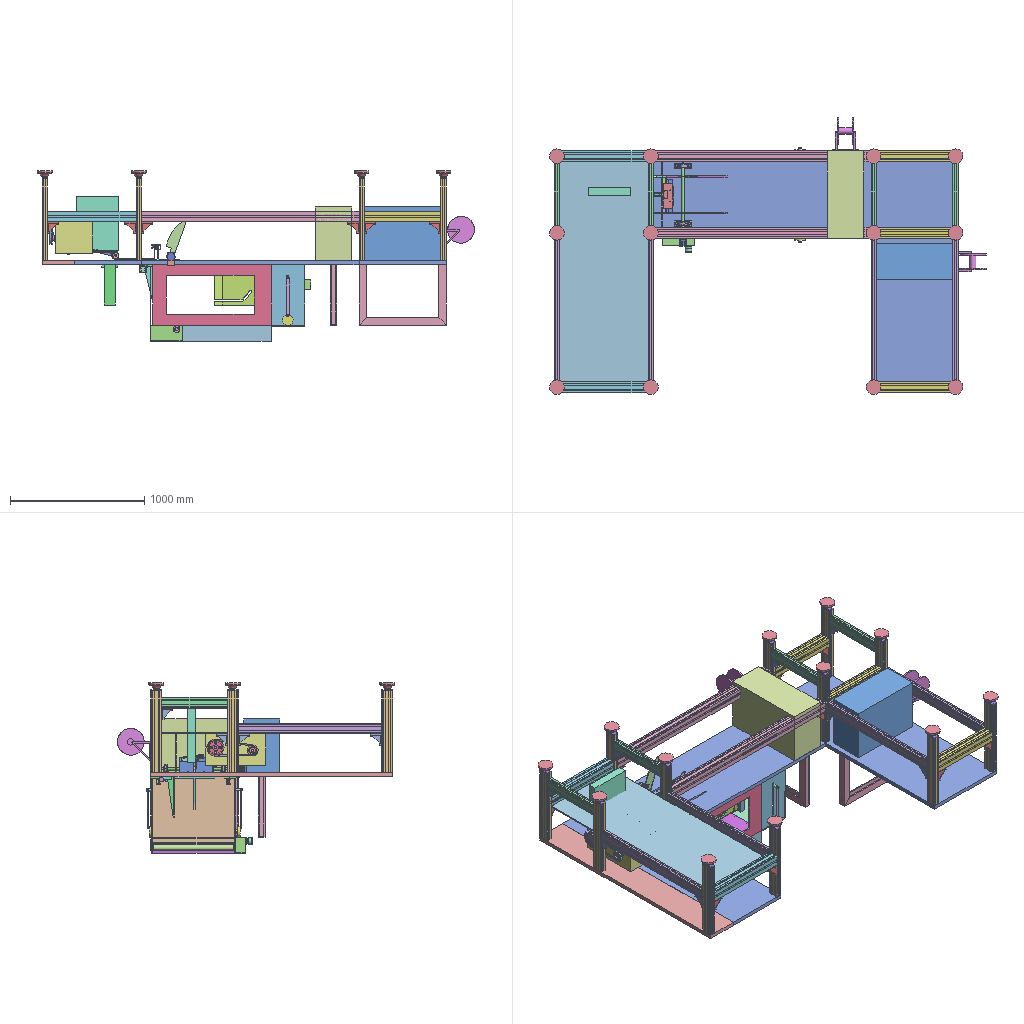Assembly | STEP file | 103 different items | 306 placed | box 3254 x 2065 x 1270 mm
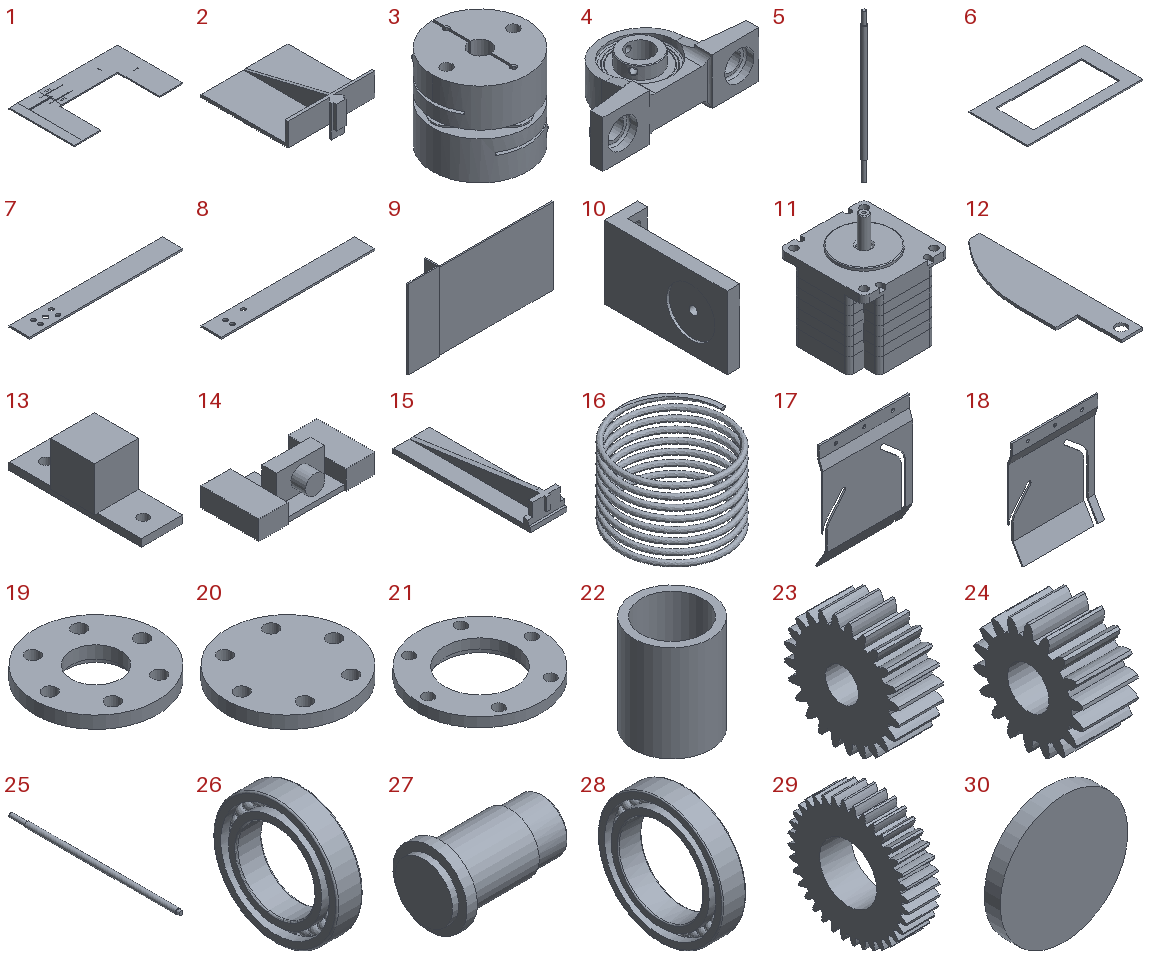Parts list (item | name | quantity | parent item | size | volume):
1 | Table top | x1 | in Assembly | 3010 x 1800 x 30 mm | 105133684 mm3
2 | tuishuban | x1 | in Assembly | 300 x 334 x 110 mm | 1327140 mm3
3 | Diaphragm coupling DEG01-D29-d6.35-e12 | x1 | in Assembly | 29 x 29 x 25.7 mm | 11994 mm3
4 | Pillow block bearing UCP204_D20 | x2 | in Assembly | 127 x 65 x 38 mm | 98212 mm3
5 | chuandongzhou | x1 | in Assembly | 20 x 20 x 596.6 mm | 161289 mm3
6 | ceban | x2 | in Assembly | 880 x 450 x 10 mm | 2061950 mm3
7 | zhiheceban1 | x1 | in Assembly | 900 x 120 x 10 mm | 1052932 mm3
8 | zhiheceban2 | x1 | in Assembly | 900 x 120 x 10 mm | 1066428 mm3
9 | zhihediban | x1 | in Assembly | 1150 x 120 x 626 mm | 7685600 mm3
10 | 57dianjijia | x1 | in Assembly | 26 x 96.5 x 57 mm | 58808 mm3
11 | 57bujindianji | x1 | in Assembly | 57 x 57 x 71.7 mm | 148752 mm3
12 | qianjiaozheban | x2 | in Assembly | 80 x 300 x 5 mm | 88356 mm3
13 | diancitie | x1 | in duizhongjigou | 30 x 90 x 35 mm | 39215 mm3
14 | duishubandingweicao | x1 | in duizhongjigou | 120 x 60 x 35 mm | 115212 mm3
15 | duizhongban | x1 | in duizhongjigou | 80 x 300 x 50 mm | 326800 mm3
16 | tanhuang | x1 | in duizhongjigou | - | 381.944 mm3
17 | gudingzhezhiban2 | x1 | in Assembly | 300 x 38.971 x 370 mm | 526356 mm3
18 | gudingzhezhiban1 | x1 | in Assembly | 300 x 39.641 x 372.5 mm | 530723 mm3
19 | zhouchenyagai1 | x4 | in Assembly | 40 x 40 x 6 mm | 4104 mm3
20 | zhouchenyagai2 | x3 | in Assembly | 40 x 40 x 6 mm | 4909 mm3
21 | zhouchenyagai3 | x1 | in Assembly | 51 x 51 x 6 mm | 5562 mm3
22 | dingjuguan | x4 | in Assembly | 20 x 20 x 25 mm | 2827 mm3
23 | spur gear_gb_GB - Spur gear 2M 24T 20PA 20FW ---S24A75H50L15.0N | x1 | in Assembly | 20 x 51.691 x 51.691 mm | 31658 mm3
24 | spur gear_gb_GB - Spur gear 2M 18T 20PA 20FW ---S18A75H50L15.0N | x2 | in Assembly | 20 x 39.557 x 40 mm | 16040 mm3
25 | tulunzhou | x1 | in Assembly | 20 x 672 x 20 mm | 200669 mm3
26 | deep groove ball bearings gb_Rolling bearings 61802 GB 276-94 | x7 | in Assembly | 5 x 24 x 24 mm | 1018 mm3
27 | zhou2 | x1 | in Assembly | 58 x 36 x 36 mm | 34937 mm3
28 | deep groove ball bearings gb_Rolling bearings 61805 GB 276-94 | x2 | in Assembly | 7 x 37 x 37 mm | 3011 mm3
29 | spur gear_gb_GB - Spur gear 2M 36T 20PA 20FW ---S36A75H50L36.0N | x1 | in Assembly | 20 x 75.809 x 75.809 mm | 59641 mm3
30 | zhoutaoφ36 | x1 | in Assembly | 48 x 9 x 48 mm | 11498 mm3
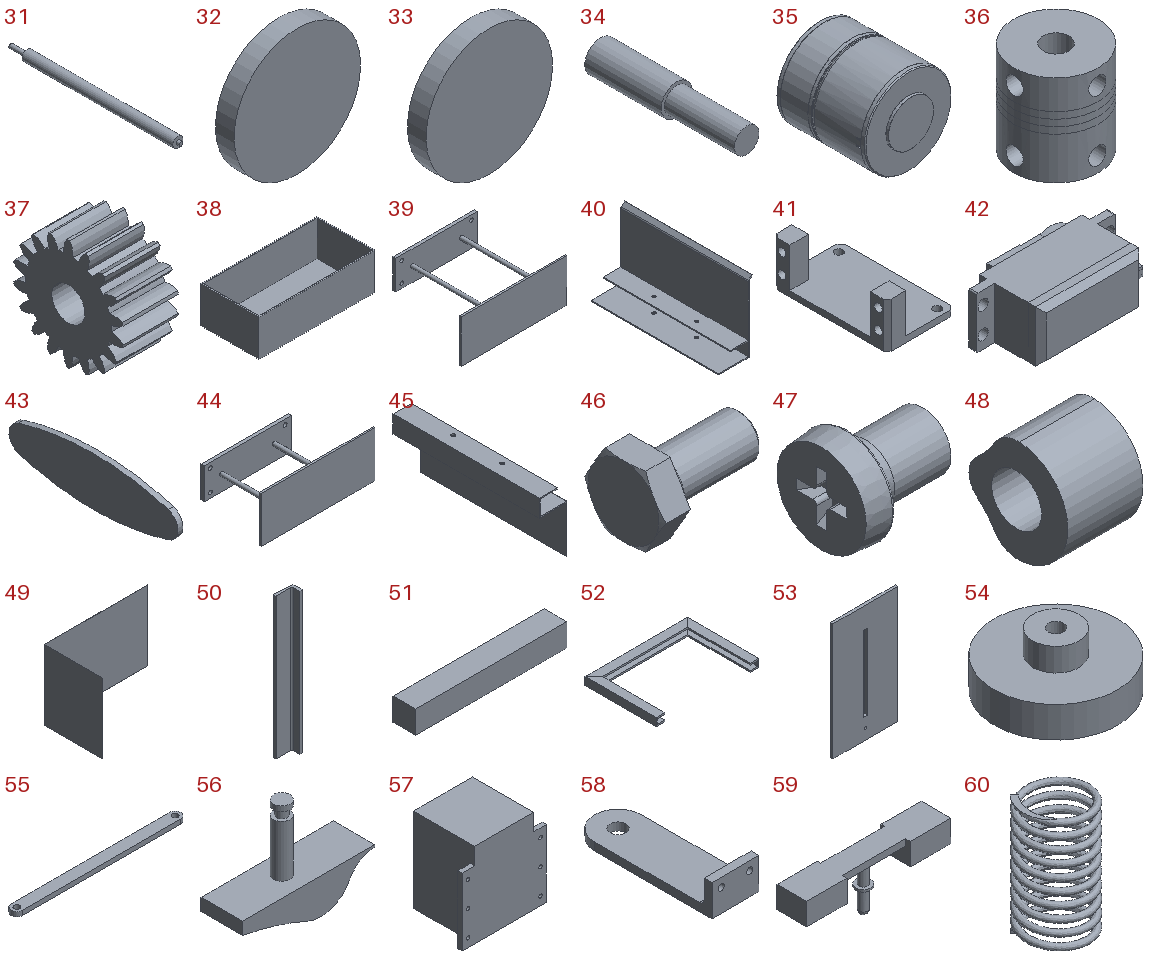31 | songzhizhou | x2 | in Assembly | 40 x 672 x 40 mm | 762386 mm3
32 | zhoutao_φ16 | x6 | in Assembly | 34 x 7 x 34 mm | 4705 mm3
33 | zhouchengai3 | x1 | in Assembly | 34 x 7 x 34 mm | 4705 mm3
34 | chilunshuruzhou | x1 | in Assembly | 15 x 71 x 15 mm | 10384 mm3
35 | zhiliudianji_Ratio 171 & 226 | x1 | in Assembly | 50 x 63.8 x 50 mm | 24472 mm3
36 | lianzhouqi | x1 | in Assembly | 19.5 x 19.5 x 21 mm | 4222 mm3
37 | spur gear_gb_GB - Spur gear 2M 18T 20PA 20FW ---S18A75H50L12.0N | x1 | in Assembly | 20 x 39.557 x 40 mm | 17312 mm3
38 | xiang | x1 | in Assembly | 240 x 120 x 75.5 mm | 239250 mm3
39 | zhijia | x1 | in zheshangye | 182 x 138 x 83.7 mm | 82026 mm3
40 | zheshangyeban | x1 | in zheshangye | 67 x 250 x 138.414 mm | 116601 mm3
41 | Servo fixing bracket-Y-middle | x2 | in Servo_left | 34.5 x 58 x 23 mm | 8576 mm3
42 | Huisheng 995 servo-Y | x2 | in Servo_left | 54 x 31.7 x 20 mm | 21472 mm3
43 | zheyetulun | x2 | in zheshangye, zhexiaye | 8 x 98.136 x 28.217 mm | 6682 mm3
44 | zhijia2 | x1 | in zhexiaye | 182 x 118 x 78.7 mm | 80895 mm3
45 | zhexiayeban | x1 | in zhexiaye | 49 x 250 x 110 mm | 92261 mm3
46 | hexagon head bolts-full thread gb_GB_FASTENER_BOLT_STBAB A M6X12-C | x8 | in zhexiaye, Assembly | 16.15 x 11.293 x 9.78 mm | 674.74 mm3
47 | cross recessed cheese head screws type a gb_GB_CROSS_SCREWS_TYPE135 M3X4-N | x10 | in zhexiaye | 5.4 x 4.982 x 4.982 mm | 52.121 mm3
48 | cuozhitulun | x1 | in Assembly | 30 x 39.5 x 40.969 mm | 25744 mm3
49 | zhi | x1 | in Assembly | 891 x 505.5 x 606 mm | 845626 mm3
50 | daozhiban | x1 | in Assembly | 80 x 45.5 x 606 mm | 689617 mm3
51 | jiazhi | x4 | in Assembly | 80 x 12 x 12 mm | 11520 mm3
52 | kunza | x2 | in Assembly | 650 x 450 x 50 mm | 1951319 mm3
53 | tieqianjijia | x1 | in Assembly | 250 x 10 x 450 mm | 1077815 mm3
54 | tieqianqubin | x2 | in Assembly | 80 x 80 x 48 mm | 111746 mm3
55 | tieqiangan | x2 | in Assembly | 300 x 20 x 8 mm | 46057 mm3
56 | tieqianhuakuai | x2 | in Assembly | 128 x 40 x 97.212 mm | 118551 mm3
57 | tieqiandianji | x2 | in Assembly | 100 x 72.5 x 123 mm | 526820 mm3
58 | tieqianzhizhu | x2 | in Assembly | 60 x 180 x 40 mm | 118454 mm3
59 | tieqiantou | x2 | in Assembly | 340 x 70 x 128 mm | 841793 mm3
60 | tieqiantanhuang | x1 | in Assembly | 21.623 x 21.623 x 40 mm | 1892 mm3
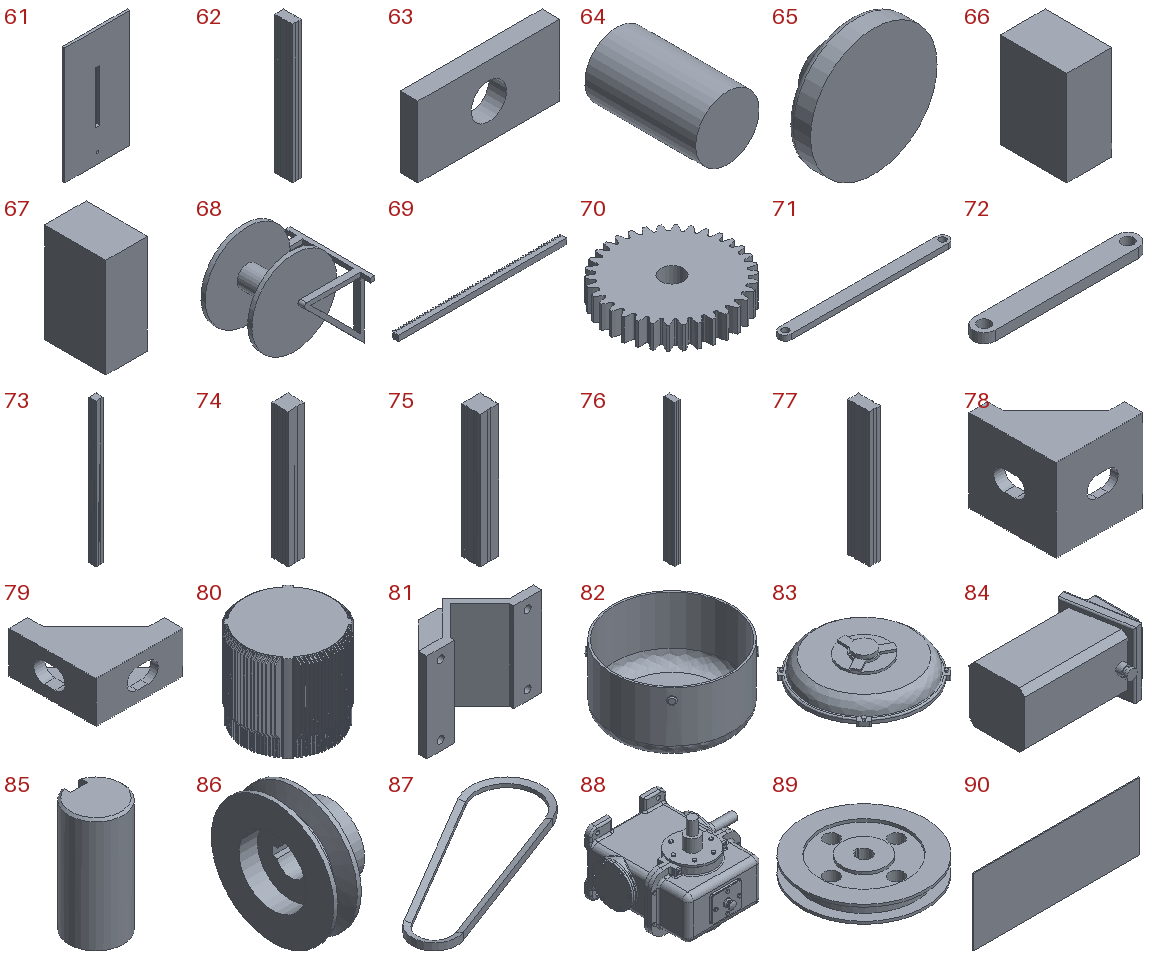61 | tieqianjijia2 | x1 | in Assembly | 250 x 10 x 450 mm | 1092215 mm3
62 | xingcai40x80x800 | x13 | in xingcaijiao | 40 x 80 x 609 mm | 1846488 mm3
63 | dianpian | x13 | in xingcaijiao | 80 x 10 x 40 mm | 28858 mm3
64 | dijiaolianjie | x13 | in xingcaijiao | 20 x 35 x 20 mm | 10996 mm3
65 | dijiao | x13 | in xingcaijiao | 110 x 46 x 110 mm | 258314 mm3
66 | kunzaxiang | x1 | in Assembly | 270 x 400 x 570 mm | 12312000 mm3
67 | kunzaxiang2 | x1 | in Assembly | 270 x 400 x 650 mm | 28248000 mm3
68 | daizhuantong | x2 | in Assembly | 250 x 200 x 250 mm | 976487 mm3
69 | rack spur rectangular_gb_GB - Rack-spur - rectangular 1.5M 20PA 10FW 10PH 300L---SAll | x2 | in Assembly | 300 x 11.5 x 10 mm | 29060 mm3
70 | Cylindrical gear 34_1.5 | x1 | in Assembly | 54 x 53.862 x 10 mm | 19460 mm3
71 | Connecting rod | x1 | in Assembly | 254.04 x 18 x 8 mm | 34769 mm3
72 | Crank | x1 | in Assembly | 136.8 x 18 x 8 mm | 17886 mm3
73 | xingcai80x80x1620 | x2 | in Assembly | 80 x 80 x 1620 mm | 10095840 mm3
74 | xingcai80x80x420 | x2 | in Assembly | 80 x 80 x 660 mm | 4113120 mm3
75 | xingcai80x80x570 | x3 | in Assembly | 80 x 80 x 570 mm | 3552240 mm3
76 | xingcai40x80x1070 | x4 | in Assembly | 40 x 80 x 1070 mm | 3244240 mm3
77 | xingcai40x80x490 | x4 | in Assembly | 40 x 80 x 490 mm | 1485680 mm3
78 | jiaoma80 | x14 | in Assembly | 84 x 84 x 80 mm | 134159 mm3
79 | jiaoma | x17 | in Assembly | 84 x 84 x 40 mm | 78299 mm3
80 | Y2_JZ_80_B_1.step 1 | x1 | in Three-phase asynchronous motor_B3_Y2-802-4_I_1 | 175 x 175 x 160 mm | 3332448 mm3
81 | Y2_DJ_80.step 2 | x1 | in Three-phase asynchronous motor_B3_Y2-802-4_I_1 | 165 x 80 x 128 mm | 452320 mm3
82 | Y2_FZ_80_1.step 3 | x1 | in Three-phase asynchronous motor_B3_Y2-802-4_I_1 | 171.5 x 171.5 x 90 mm | 182303 mm3
83 | Y2_B3_FL_80_1.step 4 | x1 | in Three-phase asynchronous motor_B3_Y2-802-4_I_1 | 157.5 x 157.5 x 35 mm | 429524 mm3
84 | Y2_JXH_80.step 5 | x1 | in Three-phase asynchronous motor_B3_Y2-802-4_I_1 | 145 x 87.322 x 78.75 mm | 651359 mm3
85 | Y2_SCZ_80_1.step 6 | x1 | in Three-phase asynchronous motor_B3_Y2-802-4_I_1 | 19 x 19 x 40 mm | 10757 mm3
86 | Plain V-belt pulley_solid wheel_A75X16X1X38X45 | x1 | in Drive structure | 38 x 80.5 x 80.5 mm | 74057 mm3
87 | Type A V-belt | x1 | in Drive structure | 354 x 224 x 12.68 mm | 82452 mm3
88 | wolunwogan | x1 | in Drive structure | 225.467 x 202.313 x 161.667 mm | 1142690 mm3
89 | dadailun | x1 | in Drive structure | 128 x 128 x 30 mm | 161160 mm3
90 | zhichenban | x1 | in Assembly | 1640 x 10 x 660 mm | 10824000 mm3
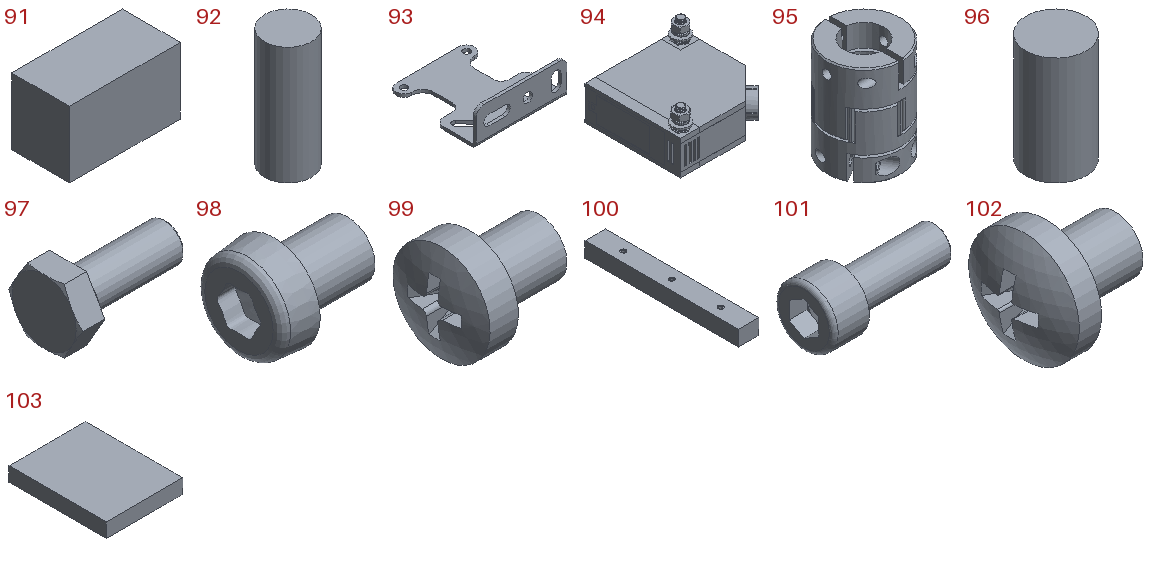91 | zhichentai | x1 | in Assembly | 450 x 234.83 x 270 mm | 28531845 mm3
92 | xiaoding | x1 | in Assembly | 10 x 10 x 25 mm | 1963 mm3
93 | guangdianzhijia | x2 | in 94 | 58 x 60 x 21.9 mm | 6452 mm3
94 | guangdiankaiguan | x2 | in 94 | - | -
95 | lianzhou | x1 | in Assembly | 30 x 30 x 40 mm | 19224 mm3
96 | xiaoding10x18 | x1 | in Assembly | 10 x 10 x 18 mm | 1414 mm3
97 | hexagon head bolts-full thread gb_GB_FASTENER_BOLT_STBAB A M4X10-N | x48 | in Assembly | 12.925 x 7.829 x 6.78 mm | 238.129 mm3
98 | hex lobular socket head cap screws-4.8 gb_GB_HEXAGON_TYPE21 M6X8-8-N | x2 | in Assembly | 11.9 x 10 x 10 mm | 475.403 mm3
99 | cross recessed small pan head screws gb_GB_CROSS_SCREWS_TYPE3 M4X5-5-N | x4 | in Assembly | 7.722 x 7 x 7 mm | 147.948 mm3
100 | lizhu | x2 | in Assembly | 40 x 300 x 30 mm | 358407 mm3
101 | hexagon socket head cap screws gb_GB_FASTENER_SCREWS_HSHCS M6X16-C | x6 | in Assembly | 22 x 10 x 10 mm | 844.992 mm3
102 | cross recessed pan head screws gb_GB_CROSS_SCREWS_TYPE1 M8X10-10  H type-N | x2 | in Assembly | 15.925 x 16 x 16 mm | 1365 mm3
103 | zhichentai2 | x1 | in Assembly | 320 x 406 x 60 mm | 7795200 mm3
Placements (level | parent | child | x y z in mm | rotation matrix by rows), first 299 of 328 lines:
1 | Assembly | Table top | -15.282 50.432 2000.0 | 1 0 0 0 1 0 0 0 1
1 | Assembly | tuishuban | -466.441 50.432 1835.0 | 0 0 -1 1 0 0 0 -1 0
1 | Assembly | Diaphragm coupling DEG01-D29-d6.35-e12 | -345.782 -270.568 2045.0 | 0.9195 0.393 0 0 0 -1 -0.393 0.9195 0
1 | Assembly | Pillow block bearing UCP204_D20 | -345.782 -164.568 2011.7 | 1 0 0 0 0 -1 0 1 0
1 | Assembly | Pillow block bearing UCP204_D20 | -345.782 265.432 2011.7 | -1 0 0 0 0 1 0 1 -0
1 | Assembly | chuandongzhou | 961.964 603.468 2400.291 | 0.5932 0.805 0 0 0 1 0.805 -0.5932 -0
1 | Assembly | ceban | -40.282 -249.568 1760.0 | -1 0 0 0 0 -1 0 -1 -0
1 | Assembly | ceban | -40.282 366.432 1760.0 | -1 0 0 0 0 -1 0 -1 -0
1 | Assembly | zhiheceban1 | -50.282 -249.568 1475.0 | 1 0 0 0 0 1 0 -1 -0
1 | Assembly | zhiheceban2 | -50.282 366.432 1475.0 | 1 0 0 0 0 1 0 -1 -0
1 | Assembly | zhihediban | -50.282 58.432 1530.0 | -1 0 0 0 0 -1 0 -1 0
1 | Assembly | 57dianjijia | -345.782 -284.568 1977.0 | 0 0 -1 1 0 0 0 -1 -0
1 | Assembly | 57bujindianji | -345.782 -335.568 2045.0 | 0 -1 0 0 0 1 -1 0 -0
1 | Assembly | qianjiaozheban | -371.292 -85.568 2032.782 | 0.9432 0.3323 0 0 0 -1 -0.3323 0.9432 0
1 | Assembly | qianjiaozheban | -371.292 186.432 2032.782 | 0.9432 0.3323 0 0 0 -1 -0.3323 0.9432 -0
1 | Assembly | duizhongjigou | -801.438 -96.846 1818.057 | 1 0 0 0 -0.01093 0.9999 0 -0.9999 -0.01093
2 | duizhongjigou | diancitie | -0.0103 -171.232 391.43 | 0 1 0 -0.01093 0 0.9999 0.9999 0 0.01093
2 | duizhongjigou | duishubandingweicao | 0.0 -170.893 360.432 | 1 0 0 0 0.01093 0.9999 0 -0.9999 0.01093
2 | duizhongjigou | duizhongban | -0.0 -20.246 302.075 | 1 0 0 0 0.9999 -0.01093 0 0.01093 0.9999
2 | duizhongjigou | tanhuang | -0.0 -150.894 360.65 | 1 0 0 0 0.9999 -0.01093 0 0.01093 0.9999
1 | Assembly | gudingzhezhiban2 | 349.718 194.852 1985.0 | 0 0 1 0 1 0 -1 0 0
1 | Assembly | gudingzhezhiban1 | 349.718 -98.988 1985.0 | 0 0 1 0 1 0 -1 0 0
1 | Assembly | zhouchenyagai1 | -294.328 -254.568 1458.0 | 0.4462 -0.8949 0 0 0 -1 0.8949 0.4462 0
1 | Assembly | zhouchenyagai2 | -294.328 371.432 1458.0 | 0.7793 0.6266 0 0 0 1 0.6266 -0.7793 -0
1 | Assembly | zhouchenyagai2 | -400.282 371.432 1458.0 | 0.935 0.3547 0 0 0 1 0.3547 -0.935 -0
1 | Assembly | zhouchenyagai2 | -400.282 371.432 1500.0 | 0.8517 0.5241 0 0 0 1 0.5241 -0.8517 -0
1 | Assembly | zhouchenyagai3 | -350.533 -254.568 1479.0 | 0.8478 0.5304 0 0 0 -1 -0.5304 0.8478 0
1 | Assembly | zhouchenyagai1 | -400.282 -254.568 1458.0 | 0.871 -0.4914 0 0 0 -1 0.4914 0.871 -0
1 | Assembly | zhouchenyagai1 | -400.282 -254.568 1500.0 | 0.9989 0.0467 0 0 0 -1 -0.0467 0.9989 -0
1 | Assembly | dingjuguan | -294.328 -271.068 1458.0 | 0.5462 -0.8377 0 0 0 1 -0.8377 -0.5462 0
1 | Assembly | dingjuguan | -400.282 -271.068 1458.0 | 1 0 0 0 0 1 0 -1 -0
1 | Assembly | dingjuguan | -400.282 -271.068 1500.0 | 1 0 0 0 0 1 0 -1 0
1 | Assembly | spur gear_gb_GB - Spur gear 2M 24T 20PA 20FW ---S24A75H50L15.0N | -294.328 -303.568 1458.0 | 0 -0.7387 -0.6741 1 0 0 0 -0.6741 0.7387
1 | Assembly | spur gear_gb_GB - Spur gear 2M 18T 20PA 20FW ---S18A75H50L15.0N | -400.282 -303.568 1458.0 | 0 -0.3057 -0.9521 1 0 0 0 -0.9521 0.3057
1 | Assembly | spur gear_gb_GB - Spur gear 2M 18T 20PA 20FW ---S18A75H50L15.0N | -400.282 -283.568 1500.0 | 0 0.9966 0.08201 -1 0 0 0 -0.08201 0.9966
1 | Assembly | tulunzhou | -294.328 368.432 1458.0 | -0.0545 0 -0.9985 0 -1 0 -0.9985 0 0.0545
1 | Assembly | deep groove ball bearings gb_Rolling bearings 61802 GB 276-94 | -294.328 365.932 1458.0 | 0 0.419 -0.908 -1 0 0 0 0.908 0.419
1 | Assembly | deep groove ball bearings gb_Rolling bearings 61802 GB 276-94 | -400.282 365.932 1500.0 | 0 -1 0 1 0 0 0 0 1
1 | Assembly | deep groove ball bearings gb_Rolling bearings 61802 GB 276-94 | -400.282 365.932 1458.0 | 0 -0.9731 -0.2304 1 0 0 0 -0.2304 0.9731
1 | Assembly | deep groove ball bearings gb_Rolling bearings 61802 GB 276-94 | -294.328 -249.068 1458.0 | 0 1 0 -1 0 0 0 0 1
1 | Assembly | deep groove ball bearings gb_Rolling bearings 61802 GB 276-94 | -400.282 -249.068 1458.0 | 0 -1 0 1 0 0 0 0 1
1 | Assembly | deep groove ball bearings gb_Rolling bearings 61802 GB 276-94 | -400.282 -249.068 1500.0 | 0 -0.9919 -0.127 1 0 0 0 -0.127 0.9919
1 | Assembly | zhou2 | -350.533 -244.568 1479.0 | 0 -0.8992 0.4375 -1 0 0 0 -0.4375 -0.8992
1 | Assembly | deep groove ball bearings gb_Rolling bearings 61805 GB 276-94 | -350.533 -290.068 1479.0 | 0 -0.06231 -0.9981 1 0 0 0 -0.9981 0.06231
1 | Assembly | deep groove ball bearings gb_Rolling bearings 61805 GB 276-94 | -350.533 -297.068 1479.0 | 0 -0.6994 -0.7147 1 0 0 0 -0.7147 0.6994
1 | Assembly | spur gear_gb_GB - Spur gear 2M 36T 20PA 20FW ---S36A75H50L36.0N | -350.533 -303.568 1479.0 | 0 0.5408 -0.8411 1 0 0 0 -0.8411 -0.5408
1 | Assembly | zhoutaoφ36 | -350.533 -309.568 1479.0 | 1 0 0 0 1 0 0 0 1
1 | Assembly | songzhizhou | -400.282 368.432 1458.0 | 0.04275 0 -0.9991 0 -1 0 -0.9991 0 -0.04275
1 | Assembly | songzhizhou | -400.282 368.432 1500.0 | -0.3236 0 -0.9462 0 -1 0 -0.9462 0 0.3236
1 | Assembly | deep groove ball bearings gb_Rolling bearings 61802 GB 276-94 | -303.768 -249.068 1506.0 | 0 -0.731 -0.6824 1 0 0 0 -0.6824 0.731
1 | Assembly | zhoutao_φ16 | -294.328 -239.568 1458.0 | 0.4406 0 -0.8977 0 -1 0 -0.8977 0 -0.4406
1 | Assembly | zhoutao_φ16 | -400.282 -239.568 1458.0 | 0.7056 0 -0.7086 0 -1 0 -0.7086 0 -0.7056
1 | Assembly | zhoutao_φ16 | -400.282 -239.568 1500.0 | 0.6086 0 -0.7935 0 -1 0 -0.7935 0 -0.6086
1 | Assembly | zhoutao_φ16 | -294.328 356.432 1458.0 | 0.9998 0 0.01816 0 1 0 -0.01816 0 0.9998
1 | Assembly | zhoutao_φ16 | -400.282 356.432 1458.0 | 1 0 0 0 1 0 0 0 1
1 | Assembly | zhoutao_φ16 | -400.282 356.432 1500.0 | 1 0 0 0 1 0 0 0 1
1 | Assembly | zhouchenyagai1 | -303.768 -254.568 1506.0 | 0.8816 0.472 0 0 0 -1 -0.472 0.8816 -0
1 | Assembly | zhouchengai3 | -303.768 -239.568 1506.0 | 0.9473 0 -0.3202 0 -1 0 -0.3202 0 -0.9473
1 | Assembly | chilunshuruzhou | -303.768 -265.068 1506.0 | 0.9582 0 -0.2862 0 1 0 0.2862 0 0.9582
1 | Assembly | zhiliudianji_Ratio 171 & 226 | -303.768 -330.068 1506.0 | 0.9582 0 -0.2862 0 1 0 0.2862 0 0.9582
1 | Assembly | lianzhouqi | -303.768 -315.068 1506.0 | 0.8979 -0.4401 0 0 0 -1 0.4401 0.8979 0
1 | Assembly | dingjuguan | -303.768 -271.068 1506.0 | 0.9977 -0.0682 0 0 0 -1 0.0682 0.9977 -0
1 | Assembly | spur gear_gb_GB - Spur gear 2M 18T 20PA 20FW ---S18A75H50L12.0N | -303.768 -283.568 1506.0 | 0 -0.5779 -0.8161 -1 0 0 0 0.8161 -0.5779
1 | Assembly | xiang | -380.282 -328.568 1475.0 | 1 0 0 0 0 1 0 -1 0
1 | Assembly | zheshangye | -290.282 59.935 1620.623 | 0 0 -1 1 0 0 0 -1 -0
2 | zheshangye | zhijia | -9.503 83.124 155.0 | 1 0 0 0 1 0 0 0 1
2 | zheshangye | zheshangyeban | -9.503 54.692 115.0 | 0 -1 0 0 0 -1 1 0 -0
2 | zheshangye | Servo_left | 16.318 -53.785 -84.102 | 0 -0.9942 0.1071 0 0.1071 0.9942 -1 0 -0
3 | Servo_left | Servo fixing bracket-Y-middle | -200.152 18.191 2.474 | 1 0 0 0 0.9942 0.1071 0 -0.1071 0.9942
3 | Servo_left | Huisheng 995 servo-Y | -196.402 18.512 5.457 | 0 -1 0 0.9942 0 0.1071 -0.1071 0 0.9942
2 | zheshangye | zheyetulun | -11.536 3.623 135.5 | 0 -0.000814 1 0 1 0.000814 -1 0 -0
1 | Assembly | zhexiaye | -285.282 50.432 2100.624 | 0 0 -1 1 0 0 0 -1 -0
2 | zhexiaye | zhijia2 | -9.503 83.124 155.0 | 1 0 0 0 1 0 0 0 1
2 | zhexiaye | zhexiayeban | -9.503 3.861 137.0 | 0 -1 0 0 0 -1 1 0 -0
2 | zhexiaye | Servo_left | -17.821 -33.785 389.102 | 0 0.9942 -0.1071 0 0.1071 0.9942 1 0 -0
3 | Servo_left | Servo fixing bracket-Y-middle | -200.152 18.191 2.474 | 1 0 0 0 0.9942 0.1071 0 -0.1071 0.9942
3 | Servo_left | Huisheng 995 servo-Y | -196.402 18.512 5.457 | 0 -1 0 0.9942 0 0.1071 -0.1071 0 0.9942
2 | zhexiaye | zheyetulun | 49.896 -13.491 169.5 | 0 0.9974 -0.07214 0 0.07214 0.9974 1 0 -0
2 | zhexiaye | hexagon head bolts-full thread gb_GB_FASTENER_BOLT_STBAB A M6X12-C | -69.503 76.474 138.0 | 0 -1 0 1 0 0 0 0 1
2 | zhexiaye | hexagon head bolts-full thread gb_GB_FASTENER_BOLT_STBAB A M6X12-C | -69.503 76.474 172.0 | 0 -1 0 1 0 0 0 0 1
2 | zhexiaye | hexagon head bolts-full thread gb_GB_FASTENER_BOLT_STBAB A M6X12-C | 50.497 76.474 172.0 | 0 -1 0 1 0 0 0 0 1
2 | zhexiaye | hexagon head bolts-full thread gb_GB_FASTENER_BOLT_STBAB A M6X12-C | 50.497 76.474 138.0 | 0 -1 0 1 0 0 0 0 1
2 | zhexiaye | cross recessed cheese head screws type a gb_GB_CROSS_SCREWS_TYPE135 M3X4-N | 25.0 -24.977 203.7 | 0 1 0 -1 0 0 0 0 1
2 | zhexiaye | cross recessed cheese head screws type a gb_GB_CROSS_SCREWS_TYPE135 M3X4-N | -25.0 -24.977 203.7 | 0 1 0 -1 0 0 0 0 1
2 | zhexiaye | cross recessed cheese head screws type a gb_GB_CROSS_SCREWS_TYPE135 M3X4-N | 24.5 -21.377 188.1 | 0 0 1 0 1 0 -1 0 -0
2 | zhexiaye | cross recessed cheese head screws type a gb_GB_CROSS_SCREWS_TYPE135 M3X4-N | 24.5 -11.377 188.1 | 0 0 1 0 1 0 -1 0 -0
2 | zhexiaye | cross recessed cheese head screws type a gb_GB_CROSS_SCREWS_TYPE135 M3X4-N | -24.5 -11.377 188.1 | 0 0 1 0 1 0 -1 0 -0
2 | zhexiaye | cross recessed cheese head screws type a gb_GB_CROSS_SCREWS_TYPE135 M3X4-N | -24.5 -21.377 188.1 | 0 0 1 0 1 0 -1 0 -0
2 | zhexiaye | cross recessed cheese head screws type a gb_GB_CROSS_SCREWS_TYPE135 M3X4-N | 24.5 -21.377 172.8 | 0 0 -1 0 1 0 1 0 0
2 | zhexiaye | cross recessed cheese head screws type a gb_GB_CROSS_SCREWS_TYPE135 M3X4-N | 24.5 -11.377 172.8 | 0 0 -1 0 1 0 1 0 0
2 | zhexiaye | cross recessed cheese head screws type a gb_GB_CROSS_SCREWS_TYPE135 M3X4-N | -24.5 -11.377 172.8 | 0 0 -1 0 1 0 1 0 0
2 | zhexiaye | cross recessed cheese head screws type a gb_GB_CROSS_SCREWS_TYPE135 M3X4-N | -24.5 -21.377 172.8 | 0 0 -1 0 1 0 1 0 0
1 | Assembly | cuozhitulun | -294.328 58.432 1458.0 | 0 -0.01108 0.9999 -1 0 0 0 -0.9999 -0.01108
1 | Assembly | zhi | -55.282 58.432 1479.0 | 1 0 0 0 0 1 0 -1 -0
1 | Assembly | daozhiban | -463.829 58.432 1493.347 | -1 0 0 0 0 -1 0 -1 -0
1 | Assembly | jiazhi | -493.282 -214.568 1979.0 | 0 0 -1 1 0 0 0 -1 -0
1 | Assembly | jiazhi | -510.209 -214.568 1979.0 | 0 0 -1 1 0 0 0 -1 -0
1 | Assembly | jiazhi | -493.282 331.432 1979.0 | 0 0 -1 1 0 0 0 -1 -0
1 | Assembly | jiazhi | -510.209 331.432 1979.0 | 0 0 1 -1 0 0 0 -1 -0
1 | Assembly | kunza | 1379.718 -449.568 1535.0 | 1 0 0 0 0 1 0 -1 0
1 | Assembly | tieqianjijia | 524.718 -249.568 1760.0 | 1 0 0 0 1 0 0 0 1
1 | Assembly | tieqianqubin | 524.718 -289.568 1575.0 | -0.9998 -0.01884 0 0 0 1 -0.01884 0.9998 0
1 | Assembly | tieqiangan | 524.115 -302.568 1606.994 | 0.002153 1 0 0 0 1 1 -0.002153 0
1 | Assembly | tieqianhuakuai | 524.718 -241.868 1890.11 | 0 -1 0 0 0 -1 1 0 0
1 | Assembly | tieqiandianji | 559.718 -239.568 1607.5 | -1 0 0 0 0 1 0 1 -0
1 | Assembly | tieqianzhizhu | 524.718 -120.238 1835.0 | -1 0 0 0 0 -1 0 -1 -0
1 | Assembly | tieqiantou | 524.718 -231.236 1835.0 | 1 0 0 0 0 1 0 -1 0
1 | Assembly | tieqiantanhuang | 524.718 -148.302 1835.0 | 0.9311 -0.3647 0 0 0 -1 0.3647 0.9311 0
1 | Assembly | tieqianjijia2 | 524.718 366.432 1760.0 | 1 0 0 0 1 0 0 0 1
1 | Assembly | xingcaijiao | 1688.464 -1386.523 3119.5 | 1 0 0 0 -1 0 0 0 -1
2 | xingcaijiao | xingcai40x80x800 | -3.747 -1.955 800.0 | 1 0 0 0 1 0 0 0 1
2 | xingcaijiao | dianpian | -3.747 -1.955 495.5 | 0 0 1 -1 0 0 0 -1 -0
2 | xingcaijiao | dijiaolianjie | -3.747 -1.955 460.5 | 1 0 0 0 0 -1 0 1 0
2 | xingcaijiao | dijiao | -3.747 -1.955 434.5 | 0.7597 0 0.6503 0.6503 0 -0.7597 0 1 -0
1 | Assembly | xingcaijiao | 1078.464 -1386.523 3119.5 | 1 0 0 0 -1 0 0 0 -1
2 | xingcaijiao | xingcai40x80x800 | -3.747 -1.955 800.0 | 1 0 0 0 1 0 0 0 1
2 | xingcaijiao | dianpian | -3.747 -1.955 495.5 | 0 0 1 -1 0 0 0 -1 -0
2 | xingcaijiao | dijiaolianjie | -3.747 -1.955 460.5 | 1 0 0 0 0 -1 0 1 0
2 | xingcaijiao | dijiao | -3.747 -1.955 434.5 | 0.7597 0 0.6503 0.6503 0 -0.7597 0 1 -0
1 | Assembly | xingcaijiao | 1078.464 -236.523 3119.5 | 1 0 0 0 -1 0 0 0 -1
2 | xingcaijiao | xingcai40x80x800 | -3.747 -1.955 800.0 | 1 0 0 0 1 0 0 0 1
2 | xingcaijiao | dianpian | -3.747 -1.955 495.5 | 0 0 1 -1 0 0 0 -1 -0
2 | xingcaijiao | dijiaolianjie | -3.747 -1.955 460.5 | 1 0 0 0 0 -1 0 1 0
2 | xingcaijiao | dijiao | -3.747 -1.955 434.5 | 0.7597 0 0.6503 0.6503 0 -0.7597 0 1 -0
1 | Assembly | xingcaijiao | 1688.464 -236.523 3119.5 | 1 0 0 0 -1 0 0 0 -1
2 | xingcaijiao | xingcai40x80x800 | -3.747 -1.955 800.0 | 1 0 0 0 1 0 0 0 1
2 | xingcaijiao | dianpian | -3.747 -1.955 495.5 | 0 0 1 -1 0 0 0 -1 -0
2 | xingcaijiao | dijiaolianjie | -3.747 -1.955 460.5 | 1 0 0 0 0 -1 0 1 0
2 | xingcaijiao | dijiao | -3.747 -1.955 434.5 | 0.7597 0 0.6503 0.6503 0 -0.7597 0 1 -0
1 | Assembly | xingcaijiao | -589.029 -1382.613 3119.5 | -1 0 0 0 1 0 0 0 -1
2 | xingcaijiao | xingcai40x80x800 | -3.747 -1.955 800.0 | 1 0 0 0 1 0 0 0 1
2 | xingcaijiao | dianpian | -3.747 -1.955 495.5 | 0 0 1 -1 0 0 0 -1 -0
2 | xingcaijiao | dijiaolianjie | -3.747 -1.955 460.5 | 1 0 0 0 0 -1 0 1 0
2 | xingcaijiao | dijiao | -3.747 -1.955 434.5 | 0.7597 0 0.6503 0.6503 0 -0.7597 0 1 -0
1 | Assembly | xingcaijiao | -589.029 337.387 3119.5 | -1 0 0 0 1 0 0 0 -1
2 | xingcaijiao | xingcai40x80x800 | -3.747 -1.955 800.0 | 1 0 0 0 1 0 0 0 1
2 | xingcaijiao | dianpian | -3.747 -1.955 495.5 | 0 0 1 -1 0 0 0 -1 -0
2 | xingcaijiao | dijiaolianjie | -3.747 -1.955 460.5 | 1 0 0 0 0 -1 0 1 0
2 | xingcaijiao | dijiao | -3.747 -1.955 434.5 | 0.7597 0 0.6503 0.6503 0 -0.7597 0 1 -0
1 | Assembly | kunzaxiang | 1379.718 -449.568 2215.0 | 0 0 -1 1 0 0 0 -1 -0
1 | Assembly | kunzaxiang2 | 864.718 50.432 2215.0 | 1 0 0 0 0 1 0 -1 0
1 | Assembly | daizhuantong | 1814.718 -389.568 2245.0 | -1 0 0 0 -1 0 0 0 1
1 | Assembly | daizhuantong | 804.718 525.432 2245.0 | 0 1 0 -1 0 0 0 0 1
1 | Assembly | rack spur rectangular_gb_GB - Rack-spur - rectangular 1.5M 20PA 10FW 10PH 300L---SAll | -766.441 45.432 2019.0 | 1 0 0 0 0 -1 0 1 -0
1 | Assembly | Cylindrical gear 34_1.5 | -760.421 55.432 2054.5 | 0.9926 0.1217 0 0 0 -1 -0.1217 0.9926 -0
1 | Assembly | rack spur rectangular_gb_GB - Rack-spur - rectangular 1.5M 20PA 10FW 10PH 300L---SAll | -1042.978 55.432 2090.0 | 1 0 0 0 0 1 0 -1 0
1 | Assembly | Connecting rod | -990.27 37.432 2108.208 | 0.9738 -0.2275 0 0 0 1 -0.2275 -0.9738 0
1 | Assembly | Crank | -1106.124 29.432 2134.5 | 0.9752 -0.2213 0 0 0 1 -0.2213 -0.9752 0
1 | Assembly | xingcaijiao | -581.536 -1386.523 3119.5 | 1 0 0 0 -1 0 0 0 -1
2 | xingcaijiao | xingcai40x80x800 | -3.747 -1.955 800.0 | 1 0 0 0 1 0 0 0 1
2 | xingcaijiao | dianpian | -3.747 -1.955 495.5 | 0 0 1 -1 0 0 0 -1 -0
2 | xingcaijiao | dijiaolianjie | -3.747 -1.955 460.5 | 1 0 0 0 0 -1 0 1 0
2 | xingcaijiao | dijiao | -3.747 -1.955 434.5 | 0.7597 0 0.6503 0.6503 0 -0.7597 0 1 -0
1 | Assembly | xingcaijiao | -1281.536 -1386.523 3119.5 | 1 0 0 0 -1 0 0 0 -1
2 | xingcaijiao | xingcai40x80x800 | -3.747 -1.955 800.0 | 1 0 0 0 1 0 0 0 1
2 | xingcaijiao | dianpian | -3.747 -1.955 495.5 | 0 0 1 -1 0 0 0 -1 -0
2 | xingcaijiao | dijiaolianjie | -3.747 -1.955 460.5 | 1 0 0 0 0 -1 0 1 0
2 | xingcaijiao | dijiao | -3.747 -1.955 434.5 | 0.7597 0 0.6503 0.6503 0 -0.7597 0 1 -0
1 | Assembly | xingcai80x80x1620 | 244.718 -234.568 2345.0 | 0 0 1 0 1 0 -1 0 0
1 | Assembly | xingcai80x80x420 | -935.282 -1384.568 2345.0 | 0 0 1 0 1 0 -1 0 0
1 | Assembly | xingcai80x80x570 | 1379.718 -1384.568 2345.0 | 0 0 1 0 1 0 -1 0 -0
1 | Assembly | xingcai40x80x1070 | 1684.718 -809.568 2345.0 | 1 0 0 0 0 1 0 -1 -0
1 | Assembly | xingcai40x80x490 | 1684.718 50.432 2536.0 | 1 0 0 0 0 1 0 -1 0
1 | Assembly | xingcaijiao | -581.536 -236.523 3119.5 | 1 0 0 0 -1 0 0 0 -1
2 | xingcaijiao | xingcai40x80x800 | -3.747 -1.955 800.0 | 1 0 0 0 1 0 0 0 1
2 | xingcaijiao | dianpian | -3.747 -1.955 495.5 | 0 0 1 -1 0 0 0 -1 -0
2 | xingcaijiao | dijiaolianjie | -3.747 -1.955 460.5 | 1 0 0 0 0 -1 0 1 0
2 | xingcaijiao | dijiao | -3.747 -1.955 434.5 | 0.7597 0 0.6503 0.6503 0 -0.7597 0 1 -0
1 | Assembly | xingcai80x80x1620 | 244.718 335.432 2345.0 | 0 0 1 0 1 0 -1 0 0
1 | Assembly | xingcai80x80x420 | -935.282 335.432 2345.0 | 0 0 1 0 1 0 -1 0 0
1 | Assembly | xingcai80x80x570 | 1379.718 335.432 2345.0 | 0 0 1 0 1 0 -1 0 -0
1 | Assembly | xingcai40x80x490 | 1074.718 50.432 2536.0 | 1 0 0 0 0 1 0 -1 0
1 | Assembly | xingcai40x80x1070 | 1074.718 -809.568 2345.0 | 1 0 0 0 0 1 0 -1 -0
1 | Assembly | xingcai40x80x490 | -585.282 50.432 2536.0 | 1 0 0 0 0 1 0 -1 0
1 | Assembly | xingcai40x80x1070 | -585.282 -809.568 2345.0 | 1 0 0 0 0 1 0 -1 -0
1 | Assembly | xingcai40x80x490 | -1285.282 50.432 2536.0 | 1 0 0 0 0 1 0 -1 0
1 | Assembly | xingcai40x80x1070 | -1285.282 -809.568 2345.0 | 1 0 0 0 0 1 0 -1 -0
1 | Assembly | jiaoma80 | -1265.282 -1344.568 2305.0 | 0 1 0 0 0 -1 -1 0 0
1 | Assembly | jiaoma | -1305.282 -1344.568 2305.0 | 0 0 1 0 1 0 -1 0 0
1 | Assembly | jiaoma80 | -605.282 -1424.568 2305.0 | 0 -1 0 0 0 1 -1 0 -0
1 | Assembly | jiaoma80 | -605.282 295.432 2305.0 | 0 -1 0 0 0 1 -1 0 -0
1 | Assembly | jiaoma80 | -1265.282 375.432 2305.0 | 0 1 0 0 0 -1 -1 0 0
1 | Assembly | jiaoma80 | 1054.718 295.432 2305.0 | 0 -1 0 0 0 1 -1 0 -0
1 | Assembly | jiaoma80 | 1664.718 295.432 2305.0 | 0 -1 0 0 0 1 -1 0 -0
1 | Assembly | jiaoma | 1054.718 -1344.568 2305.0 | 0 0 1 0 1 0 -1 0 0
1 | Assembly | jiaoma | 1664.718 -1344.568 2305.0 | 0 0 1 0 1 0 -1 0 0
1 | Assembly | jiaoma80 | 1664.718 -1424.568 2305.0 | 0 -1 0 0 0 1 -1 0 -0
1 | Assembly | jiaoma80 | 1094.718 -1344.568 2305.0 | 0 1 0 0 0 -1 -1 0 0
1 | Assembly | kunza | 864.718 50.432 1535.0 | 0 0 1 -1 0 0 0 -1 -0
1 | Assembly | Drive structure | -1051.742 -189.273 2623.496 | -1 0 0 0 0 -1 0 -1 -0
2 | Drive structure | Three-phase asynchronous motor_B3_Y2-802-4_I_1 | 45.716 442.329 193.169 | 0 0 1 0 1 0 -1 0 -0
3 | Three-phase asynchronous motor_B3_Y2-802-4_I_1 | Y2_JZ_80_B_1.step 1 | -0.0 0.0 -0.0 | 1 0 0 0 1 0 0 0 1
3 | Three-phase asynchronous motor_B3_Y2-802-4_I_1 | Y2_DJ_80.step 2 | -0.0 0.0 -0.0 | 1 0 0 0 1 0 0 0 1
3 | Three-phase asynchronous motor_B3_Y2-802-4_I_1 | Y2_FZ_80_1.step 3 | -0.0 0.0 -0.0 | 1 0 0 0 1 0 0 0 1
3 | Three-phase asynchronous motor_B3_Y2-802-4_I_1 | Y2_B3_FL_80_1.step 4 | -0.0 0.0 -0.0 | 1 0 0 0 1 0 0 0 1
3 | Three-phase asynchronous motor_B3_Y2-802-4_I_1 | Y2_JXH_80.step 5 | -0.0 0.0 -0.0 | 1 0 0 0 1 0 0 0 1
3 | Three-phase asynchronous motor_B3_Y2-802-4_I_1 | Y2_SCZ_80_1.step 6 | -0.0 0.0 -0.0 | 1 0 0 0 1 0 0 0 1
2 | Drive structure | Plain V-belt pulley_solid wheel_A75X16X1X38X45 | 197.716 442.329 193.169 | -1 0 0 0 1 0 0 0 -1
2 | Drive structure | Type A V-belt | 188.716 442.329 193.169 | 0 0 1 -0.4986 0.8668 0 -0.8668 -0.4986 0
2 | Drive structure | wolunwogan | -27.284 488.996 -135.038 | 1 0 0 0 -1 0 0 0 -1
2 | Drive structure | dadailun | 188.716 421.7 -83.371 | 0 0 1 0 1 0 -1 0 0
1 | Assembly | xingcaijiao | -1281.536 333.477 3119.5 | 1 0 0 0 -1 0 0 0 -1
2 | xingcaijiao | xingcai40x80x800 | -3.747 -1.955 800.0 | 1 0 0 0 1 0 0 0 1
2 | xingcaijiao | dianpian | -3.747 -1.955 495.5 | 0 0 1 -1 0 0 0 -1 -0
2 | xingcaijiao | dijiaolianjie | -3.747 -1.955 460.5 | 1 0 0 0 0 -1 0 1 0
2 | xingcaijiao | dijiao | -3.747 -1.955 434.5 | 0.7597 0 0.6503 0.6503 0 -0.7597 0 1 -0
1 | Assembly | xingcaijiao | -1281.536 -236.523 3119.5 | 1 0 0 0 -1 0 0 0 -1
2 | xingcaijiao | xingcai40x80x800 | -3.747 -1.955 800.0 | 1 0 0 0 1 0 0 0 1
2 | xingcaijiao | dianpian | -3.747 -1.955 495.5 | 0 0 1 -1 0 0 0 -1 -0
2 | xingcaijiao | dijiaolianjie | -3.747 -1.955 460.5 | 1 0 0 0 0 -1 0 1 0
2 | xingcaijiao | dijiao | -3.747 -1.955 434.5 | 0.7597 0 0.6503 0.6503 0 -0.7597 0 1 -0
1 | Assembly | jiaoma | -1305.282 -194.568 2305.0 | 0 0 1 0 1 0 -1 0 0
1 | Assembly | jiaoma | -605.282 -1344.568 2305.0 | 0 0 1 0 1 0 -1 0 0
1 | Assembly | jiaoma | -1265.282 -274.568 2305.0 | 0 0 -1 0 -1 0 -1 0 0
1 | Assembly | jiaoma | -1265.282 295.432 2496.0 | 0 0 -1 0 -1 0 -1 0 0
1 | Assembly | jiaoma | -565.282 295.432 2496.0 | 0 0 -1 0 -1 0 -1 0 0
1 | Assembly | jiaoma | -605.282 -194.568 2305.0 | 0 0 1 0 1 0 -1 0 0
1 | Assembly | jiaoma | -565.282 -274.568 2305.0 | 0 0 -1 0 -1 0 -1 0 0
1 | Assembly | jiaoma80 | 1094.718 -194.568 2305.0 | 0 1 0 0 0 -1 -1 0 0
1 | Assembly | jiaoma80 | 1664.718 -274.568 2305.0 | 0 -1 0 0 0 1 -1 0 -0
1 | Assembly | jiaoma80 | 1094.718 375.432 2305.0 | 0 1 0 0 0 -1 -1 0 0
1 | Assembly | jiaoma | 1054.718 -1344.568 2305.0 | 0 0 1 0 1 0 -1 0 0
1 | Assembly | jiaoma | 1094.718 295.432 2496.0 | 0 0 -1 0 -1 0 -1 0 0
1 | Assembly | jiaoma | 1094.718 -274.568 2305.0 | 0 0 -1 0 -1 0 -1 0 0
1 | Assembly | jiaoma | 1054.718 -194.568 2305.0 | 0 0 1 0 1 0 -1 0 0
1 | Assembly | jiaoma80 | 1054.718 -274.568 2305.0 | 0 -1 0 0 0 1 -1 0 -0
1 | Assembly | jiaoma | 1704.718 295.432 2496.0 | 0 0 -1 0 -1 0 -1 0 0
1 | Assembly | jiaoma | 1664.718 -194.568 2305.0 | 0 0 1 0 1 0 -1 0 0
1 | Assembly | jiaoma | 1704.718 -274.568 2305.0 | 0 0 -1 0 -1 0 -1 0 0
1 | Assembly | jiaoma80 | -565.282 375.432 2305.0 | 0 1 0 0 0 -1 -1 0 0
1 | Assembly | jiaoma80 | -565.282 -194.568 2305.0 | 0 1 0 0 0 -1 -1 0 0
1 | Assembly | xingcai80x80x570 | 1379.718 -234.568 2345.0 | 0 0 1 0 1 0 -1 0 -0
1 | Assembly | zhichenban | -935.282 -524.568 2305.0 | 0 0 1 1 0 0 0 1 0
1 | Assembly | zhichentai | -1202.457 -479.942 2187.585 | 0 0 1 1 0 0 0 1 0
1 | Assembly | xiaoding | -1106.124 37.432 2134.5 | 0.9999 -0.01701 0 0 0 -1 0.01701 0.9999 -0
1 | Assembly | guangdiankaiguan | -553.26 264.682 1953.778 | 1 0 0 0 0 1 0 -1 -0
2 | guangdiankaiguan | guangdianzhijia | 0.9773 -31.222 60.0 | 1 0 0 0 1 0 0 0 1
2 | guangdiankaiguan | guangdiankaiguan | 0.6765 -2.124 50.85 | -1 0 0 0 1 0 0 0 -1
1 | Assembly | lianzhou | -1106.124 3.432 2134.5 | -0.1568 0.9876 0 0 0 -1 -0.9876 -0.1568 -0
1 | Assembly | xiaoding10x18 | -760.421 46.432 2054.5 | 0.8671 -0.4981 0 0 0 -1 0.4981 0.8671 -0
1 | Assembly | hexagon head bolts-full thread gb_GB_FASTENER_BOLT_STBAB A M4X10-N | -286.05 -261.493 1445.491 | 0 -1 0 1 0 0 0 0 1
1 | Assembly | hexagon head bolts-full thread gb_GB_FASTENER_BOLT_STBAB A M4X10-N | -279.356 -261.493 1458.915 | 0 -1 0 1 0 0 0 0 1
1 | Assembly | hexagon head bolts-full thread gb_GB_FASTENER_BOLT_STBAB A M4X10-N | -301.022 -261.493 1444.576 | 0 -1 0 1 0 0 0 0 1
1 | Assembly | hexagon head bolts-full thread gb_GB_FASTENER_BOLT_STBAB A M4X10-N | -309.3 -261.493 1457.085 | 0 -1 0 1 0 0 0 0 1
1 | Assembly | hexagon head bolts-full thread gb_GB_FASTENER_BOLT_STBAB A M4X10-N | -287.635 -261.493 1471.424 | 0 -1 0 1 0 0 0 0 1
1 | Assembly | hexagon head bolts-full thread gb_GB_FASTENER_BOLT_STBAB A M4X10-N | -302.607 -261.493 1470.509 | 0 -1 0 1 0 0 0 0 1
1 | Assembly | hexagon head bolts-full thread gb_GB_FASTENER_BOLT_STBAB A M4X10-N | -351.295 -261.493 1457.514 | 0 -1 0 1 0 0 0 0 1
1 | Assembly | hexagon head bolts-full thread gb_GB_FASTENER_BOLT_STBAB A M4X10-N | -332.306 -261.493 1467.597 | 0 -1 0 1 0 0 0 0 1
1 | Assembly | hexagon head bolts-full thread gb_GB_FASTENER_BOLT_STBAB A M4X10-N | -369.522 -261.493 1468.917 | 0 -1 0 1 0 0 0 0 1
1 | Assembly | hexagon head bolts-full thread gb_GB_FASTENER_BOLT_STBAB A M4X10-N | -400.432 -261.493 1443.001 | 0 -1 0 1 0 0 0 0 1
1 | Assembly | hexagon head bolts-full thread gb_GB_FASTENER_BOLT_STBAB A M4X10-N | -387.367 -261.493 1450.371 | 0 -1 0 1 0 0 0 0 1
1 | Assembly | hexagon head bolts-full thread gb_GB_FASTENER_BOLT_STBAB A M4X10-N | -413.347 -261.493 1450.63 | 0 -1 0 1 0 0 0 0 1
1 | Assembly | hexagon head bolts-full thread gb_GB_FASTENER_BOLT_STBAB A M4X10-N | -413.198 -261.493 1465.629 | 0 -1 0 1 0 0 0 0 1
1 | Assembly | hexagon head bolts-full thread gb_GB_FASTENER_BOLT_STBAB A M4X10-N | -400.133 -261.493 1472.999 | 0 -1 0 1 0 0 0 0 1
1 | Assembly | hexagon head bolts-full thread gb_GB_FASTENER_BOLT_STBAB A M4X10-N | -393.397 -261.493 1486.674 | 0 -1 0 1 0 0 0 0 1
1 | Assembly | hexagon head bolts-full thread gb_GB_FASTENER_BOLT_STBAB A M4X10-N | -408.381 -261.493 1487.374 | 0 -1 0 1 0 0 0 0 1
1 | Assembly | hexagon head bolts-full thread gb_GB_FASTENER_BOLT_STBAB A M4X10-N | -415.266 -261.493 1500.7 | 0 -1 0 1 0 0 0 0 1
1 | Assembly | hexagon head bolts-full thread gb_GB_FASTENER_BOLT_STBAB A M4X10-N | -407.168 -261.493 1513.326 | 0 -1 0 1 0 0 0 0 1
1 | Assembly | hexagon head bolts-full thread gb_GB_FASTENER_BOLT_STBAB A M4X10-N | -385.299 -261.493 1499.3 | 0 -1 0 1 0 0 0 0 1
1 | Assembly | hexagon head bolts-full thread gb_GB_FASTENER_BOLT_STBAB A M4X10-N | -368.76 -261.493 1490.403 | 0 -1 0 1 0 0 0 0 1
1 | Assembly | hexagon head bolts-full thread gb_GB_FASTENER_BOLT_STBAB A M4X10-N | -392.184 -261.493 1512.626 | 0 -1 0 1 0 0 0 0 1
1 | Assembly | hexagon head bolts-full thread gb_GB_FASTENER_BOLT_STBAB A M4X10-N | -290.544 -261.493 1498.92 | 0 -1 0 1 0 0 0 0 1
1 | Assembly | hexagon head bolts-full thread gb_GB_FASTENER_BOLT_STBAB A M4X10-N | -303.287 -261.493 1491.008 | 0 -1 0 1 0 0 0 0 1
1 | Assembly | hexagon head bolts-full thread gb_GB_FASTENER_BOLT_STBAB A M4X10-N | -316.992 -261.493 1513.08 | 0 -1 0 1 0 0 0 0 1
1 | Assembly | hexagon head bolts-full thread gb_GB_FASTENER_BOLT_STBAB A M4X10-N | -291.024 -261.493 1513.912 | 0 -1 0 1 0 0 0 0 1
1 | Assembly | hexagon head bolts-full thread gb_GB_FASTENER_BOLT_STBAB A M4X10-N | -304.248 -261.493 1520.992 | 0 -1 0 1 0 0 0 0 1
1 | Assembly | hexagon head bolts-full thread gb_GB_FASTENER_BOLT_STBAB A M4X10-N | -349.771 -261.493 1500.486 | 0 -1 0 1 0 0 0 0 1
1 | Assembly | hexagon head bolts-full thread gb_GB_FASTENER_BOLT_STBAB A M4X10-N | -316.511 -261.493 1498.088 | 0 -1 0 1 0 0 0 0 1
1 | Assembly | hexagon head bolts-full thread gb_GB_FASTENER_BOLT_STBAB A M4X10-N | -331.544 -261.493 1489.083 | 0 -1 0 1 0 0 0 0 1
1 | Assembly | hexagon head bolts-full thread gb_GB_FASTENER_BOLT_STBAB A M4X10-N | -387.218 -261.493 1465.37 | 0 -1 0 1 0 0 0 0 1
1 | Assembly | hexagon head bolts-full thread gb_GB_FASTENER_BOLT_STBAB A M4X10-N | -280.343 378.357 1452.576 | 0 1 0 -1 0 0 0 0 1
1 | Assembly | hexagon head bolts-full thread gb_GB_FASTENER_BOLT_STBAB A M4X10-N | -292.033 378.357 1443.177 | 0 1 0 -1 0 0 0 0 1
1 | Assembly | hexagon head bolts-full thread gb_GB_FASTENER_BOLT_STBAB A M4X10-N | -306.018 378.357 1448.601 | 0 1 0 -1 0 0 0 0 1
1 | Assembly | hexagon head bolts-full thread gb_GB_FASTENER_BOLT_STBAB A M4X10-N | -308.313 378.357 1463.424 | 0 1 0 -1 0 0 0 0 1
1 | Assembly | hexagon head bolts-full thread gb_GB_FASTENER_BOLT_STBAB A M4X10-N | -296.623 378.357 1472.823 | 0 1 0 -1 0 0 0 0 1
1 | Assembly | hexagon head bolts-full thread gb_GB_FASTENER_BOLT_STBAB A M4X10-N | -282.638 378.357 1467.399 | 0 1 0 -1 0 0 0 0 1
1 | Assembly | hexagon head bolts-full thread gb_GB_FASTENER_BOLT_STBAB A M4X10-N | -388.662 378.357 1448.515 | 0 1 0 -1 0 0 0 0 1
1 | Assembly | hexagon head bolts-full thread gb_GB_FASTENER_BOLT_STBAB A M4X10-N | -386.258 378.357 1463.321 | 0 1 0 -1 0 0 0 0 1
1 | Assembly | hexagon head bolts-full thread gb_GB_FASTENER_BOLT_STBAB A M4X10-N | -402.687 378.357 1443.194 | 0 1 0 -1 0 0 0 0 1
1 | Assembly | hexagon head bolts-full thread gb_GB_FASTENER_BOLT_STBAB A M4X10-N | -414.307 378.357 1452.679 | 0 1 0 -1 0 0 0 0 1
1 | Assembly | hexagon head bolts-full thread gb_GB_FASTENER_BOLT_STBAB A M4X10-N | -411.903 378.357 1467.485 | 0 1 0 -1 0 0 0 0 1
1 | Assembly | hexagon head bolts-full thread gb_GB_FASTENER_BOLT_STBAB A M4X10-N | -397.878 378.357 1472.806 | 0 1 0 -1 0 0 0 0 1
1 | Assembly | hexagon head bolts-full thread gb_GB_FASTENER_BOLT_STBAB A M4X10-N | -387.087 378.357 1492.867 | 0 1 0 -1 0 0 0 0 1
1 | Assembly | hexagon head bolts-full thread gb_GB_FASTENER_BOLT_STBAB A M4X10-N | -399.862 378.357 1485.006 | 0 1 0 -1 0 0 0 0 1
1 | Assembly | hexagon head bolts-full thread gb_GB_FASTENER_BOLT_STBAB A M4X10-N | -413.058 378.357 1492.139 | 0 1 0 -1 0 0 0 0 1
1 | Assembly | hexagon head bolts-full thread gb_GB_FASTENER_BOLT_STBAB A M4X10-N | -413.478 378.357 1507.133 | 0 1 0 -1 0 0 0 0 1
1 | Assembly | hexagon head bolts-full thread gb_GB_FASTENER_BOLT_STBAB A M4X10-N | -400.703 378.357 1514.994 | 0 1 0 -1 0 0 0 0 1
1 | Assembly | hexagon head bolts-full thread gb_GB_FASTENER_BOLT_STBAB A M4X10-N | -387.507 378.357 1507.861 | 0 1 0 -1 0 0 0 0 1
1 | Assembly | hexagon head bolts-full thread gb_GB_FASTENER_BOLT_STBAB A M6X12-C | -462.282 -9.568 1544.15 | 0 0 1 0 1 0 -1 0 0
1 | Assembly | hexagon head bolts-full thread gb_GB_FASTENER_BOLT_STBAB A M6X12-C | -428.282 -9.568 1544.15 | 0 0 1 0 1 0 -1 0 0
1 | Assembly | hexagon head bolts-full thread gb_GB_FASTENER_BOLT_STBAB A M6X12-C | -462.282 110.432 1544.15 | 0 0 1 0 1 0 -1 0 0
1 | Assembly | hexagon head bolts-full thread gb_GB_FASTENER_BOLT_STBAB A M6X12-C | -428.282 110.432 1544.15 | 0 0 1 0 1 0 -1 0 0
1 | Assembly | xingcaijiao | 1078.464 333.477 3119.5 | 1 0 0 0 -1 0 0 0 -1
2 | xingcaijiao | xingcai40x80x800 | -3.747 -1.955 800.0 | 1 0 0 0 1 0 0 0 1
2 | xingcaijiao | dianpian | -3.747 -1.955 495.5 | 0 0 1 -1 0 0 0 -1 -0
2 | xingcaijiao | dijiaolianjie | -3.747 -1.955 460.5 | 1 0 0 0 0 -1 0 1 0
2 | xingcaijiao | dijiao | -3.747 -1.955 434.5 | 0.7597 0 0.6503 0.6503 0 -0.7597 0 1 -0
1 | Assembly | xingcaijiao | 1688.464 333.477 3119.5 | 1 0 0 0 -1 0 0 0 -1
2 | xingcaijiao | xingcai40x80x800 | -3.747 -1.955 800.0 | 1 0 0 0 1 0 0 0 1